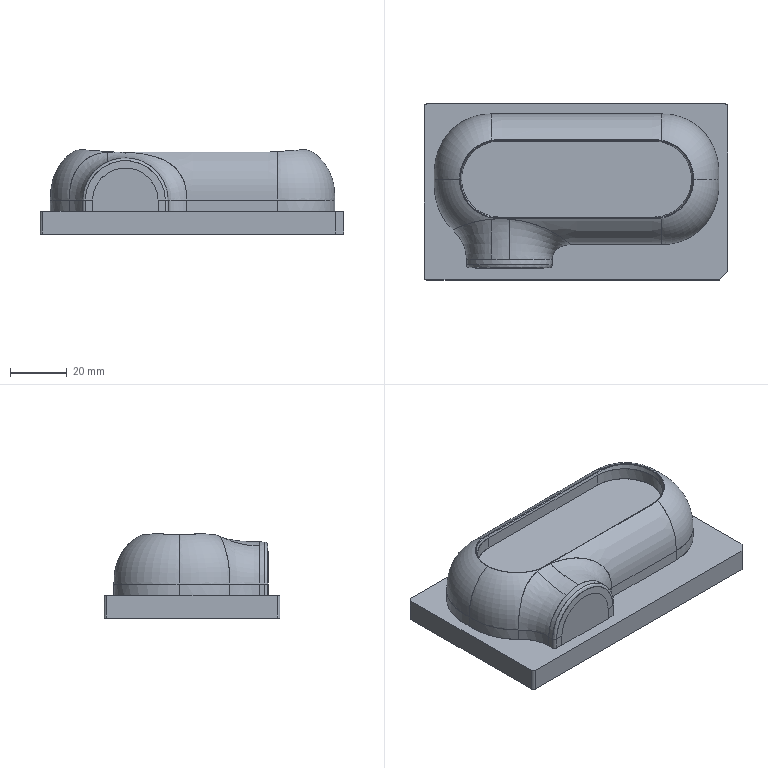NC program | PowerMill | posted by the shop | part box 107 x 62 x 29.663 mm
Lines 1 to 1401 of 415021:
%
G40 G49 G17 G80
( TOOL ID   D10C_1_1_1 )
( TOOL DIA. 10. TIP RAD 0 LENGTH 85.12 )
( Z = -.028 )
T1 M6
T3
G91 G28 Z0
G0 G90 G54
M08
S8000 M3
G0 X0 Y0 M8
G43 Z10.2 H1
X61.32 Y33.82
Z1.172
G1 Z-.028 F6000
X56.32 F10000
X-56.32
Y28.183
X56.32
Y22.547
X-56.32
Y16.91
X56.32
Y11.273
X-56.32
Y5.637
X56.32
Y0
X-56.32
Y-5.637
X56.32
Y-11.273
X-56.32
Y-16.91
X56.32
Y-22.547
X-56.32
Y-28.183
X56.32
Y-33.82
X-56.32
X-61.32
G0 Z10.2
X.218 Y.346
Z9.922
X-63.011 Y-.592
Z.741
G1 Z-.459 F6000
X-62.484 F10000
G3 X-57.736 Y4.155 I0 J4.747
G1 Y34.32
G2 X-56.736 Y35.32 I1. J0
G1 X57.172
G2 X58.172 Y34.32 I0 J-1.
G1 Y4.157
X46.989 Y4.213
X46.981 Y2.666
X46.858 Y1.119
X46.75 Y.346
X46.444 Y-1.201
X46.234 Y-1.974
X45.989 Y-2.748
X45.705 Y-3.521
X45.379 Y-4.295
X44.69 Y-5.67
X43.917 Y-6.909
X43.143 Y-7.943
X42.37 Y-8.824
X41.464 Y-9.709
X40.538 Y-10.482
X39.276 Y-11.364
X38.103 Y-12.029
X36.956 Y-12.564
X36.336 Y-12.802
X35.409 Y-13.113
X34.635 Y-13.324
X33.862 Y-13.484
X33.089 Y-13.541
X32.315 Y-13.482
X31.542 Y-13.336
X30.768 Y-13.065
X30.255 Y-12.802
X29.995 Y-12.641
X29.221 Y-12.006
X28.448 Y-11.061
X28.137 Y-10.482
X27.854 Y-9.709
X27.701 Y-8.935
X27.663 Y-8.162
X27.738 Y-7.388
X27.938 Y-6.615
X28.277 Y-5.841
X28.448 Y-5.53
X28.775 Y-5.068
X29.221 Y-4.565
X29.519 Y-4.295
X29.995 Y-3.932
X30.618 Y-3.521
X31.542 Y-2.947
X32.315 Y-2.422
X33.089 Y-1.791
X33.676 Y-1.201
X34.287 Y-.427
X34.635 Y.09
X35.16 Y1.119
X35.409 Y1.758
X35.658 Y2.666
X35.791 Y3.44
X35.867 Y4.213
X35.856 Y4.987
X35.767 Y5.76
X35.614 Y6.533
X35.386 Y7.307
X35.076 Y8.08
X34.67 Y8.854
X34.149 Y9.627
X33.488 Y10.401
X33.089 Y10.791
X32.315 Y11.421
X31.542 Y11.949
X31.531 Y11.956
X30.768 Y12.422
X29.995 Y12.931
X29.296 Y13.494
X28.632 Y14.268
X28.448 Y14.531
X28.326 Y14.758
X23.408 Y12.411
X18.896 Y10.258
X13.458 Y8.694
X7.5 Y6.981
X2.145 Y5.441
G3 X.47 Y6.699 I-1.67 J-.48
G1 X-.091 Y6.697
G3 X-1.804 Y4.698 I.005 J-1.738
G1 X-.811 Y-1.952
G3 X1.364 Y-1.929 I1.086 J.159
G1 X2.2 Y4.745
G3 X2.145 Y5.441 I-1.724 J.216
G1 X7.5 Y6.981
X6.371 Y11.317
G3 X4.434 Y12.813 I-1.935 J-.504
G1 X-4.065 Y12.807
G3 X-6.001 Y11.304 I.001 J-2.
G1 X-7.581 Y5.143
G3 X-7.603 Y4.242 I1.937 J-.497
G1 X-6.958 Y1.11
G2 X-5.807 Y-7.803 I-58.994 J-12.149
G1 X-5.648 Y-10.764
G3 X-3.648 Y-12.657 I1.997 J.107
G1 X4.075 Y-12.647
G3 X6.072 Y-10.669 I-.003 J2.
G1 X6.082 Y-9.832
G2 X6.632 Y-4.073 I34.451 J-.385
G1 X8.091 Y3.977
G3 X8.058 Y4.837 I-1.968 J.357
G1 X7.5 Y6.981
X13.458 Y8.694
X13.328 Y9.066
G2 X11.725 Y15.34 I35.2 J12.336
G1 X11.424 Y17.169
G3 X9.45 Y18.844 I-1.973 J-.325
G1 X-9.045 Y18.838
G3 X-11.014 Y17.186 I.001 J-2.
G1 X-11.379 Y15.118
G2 X-12.836 Y9.467 I-37.025 J6.534
G1 X-14.269 Y5.285
G3 X-14.267 Y3.984 I1.892 J-.648
G1 X-12.599 Y-.845
G2 X-12.515 Y-15.174 I-21.097 J-7.289
G1 X-12.73 Y-15.823
G3 X-10.831 Y-18.454 I1.898 J-.631
G1 X11.141 Y-18.441
G3 X13.074 Y-15.933 I-.001 J2.
G1 X12.52 Y-13.822
G2 X12.157 Y-4.693 I20.543 J5.389
G1 X12.185 Y-4.537
G2 X12.999 Y-1.397 I20.789 J-3.718
G1 X14.751 Y3.705
G3 X14.747 Y5.016 I-1.892 J.65
G1 X13.458 Y8.694
X18.896 Y10.258
G2 X19.274 Y24.679 I14.332 J6.839
G1 X19.284 Y24.697
Y24.699
X19.282 Y24.7
X-18.832
X-18.834 Y24.699
Y24.697
X-18.825 Y24.679
X-18.78 Y24.596
X-18.736 Y24.512
X-18.735 Y24.51
G2 X-23.208 Y4.655 I-13.944 J-7.29
G1 X-23.224 Y4.643
X-23.225 Y4.641
X-23.224 Y4.639
X-23.21 Y4.628
G2 X-39.737 Y-22.434 I-9.627 J-12.698
G1 X-41.719 Y-21.482
G2 X-47.231 Y-17.93 I11.424 J23.781
G1 X-47.249 Y-17.915
X-47.25
X-47.251 Y-17.917
X-47.16 Y-24.004
X-47.159 Y-24.007
X-47.157 Y-24.008
X30.537
X30.538 Y-24.007
Y-24.005
X30.52 Y-24.002
G2 X23.708 Y-21.091 I2.631 J15.581
X17.688 Y-5.165 I9.443 J12.67
G1 X17.714 Y-5.041
G2 X23.758 Y4.324 I15.259 J-3.214
G1 X23.773 Y4.335
X23.774 Y4.337
X23.773 Y4.339
X23.756 Y4.351
G2 X18.896 Y10.258 I9.472 J12.746
G1 X23.408 Y12.411
G3 X27.403 Y7.907 I9.82 J4.686
G1 X27.843 Y7.628
G2 X27.815 Y1.013 I-2.091 J-3.299
G1 X27.377 Y.74
G3 X22.606 Y-6.072 I5.597 J-8.996
G1 X22.58 Y-6.195
G3 X38.305 Y-17.914 I10.57 J-2.227
G1 X40.991 Y-16.456
G3 X50.325 Y-6.291 I-10.147 J18.686
G1 X50.81 Y-5.184
G2 X52.872 Y-5.631 I.986 J-.431
G1 X52.551 Y-27.037
G2 X50.551 Y-29.007 I-2. J.03
G1 X41.678
Y-24.008
X35.763
X35.762 Y-24.007
X35.763 Y-24.005
X35.781 Y-24.002
G3 X40.691 Y-22.308 I-2.63 J15.581
G1 X43.377 Y-20.849
G3 X47.665 Y-17.938 I-12.532 J23.079
G1 X47.685 Y-17.922
X47.687
Y-17.924
X47.596 Y-24.004
X47.595 Y-24.007
X47.593 Y-24.008
X41.678
Y-29.007
X-50.115
G2 X-52.115 Y-27.037 I0 J2.
G1 X-52.436 Y-5.602
G2 X-50.373 Y-5.155 I1.076 J.016
G1 X-49.889 Y-6.262
G3 X-39.554 Y-16.976 I19.595 J8.562
G1 X-37.573 Y-17.927
G3 X-27.019 Y1.189 I4.735 J9.857
G1 X-27.459 Y1.466
G2 X-27.446 Y7.832 I1.998 J3.179
G1 X-27.007 Y8.105
G3 X-36.928 Y27.079 I-5.673 J9.115
G1 X-38.994 Y26.189
G3 X-49.886 Y15.391 I8.303 J-19.269
G1 X-50.373 Y14.289
G2 X-52.436 Y14.75 I-.986 J.435
G1 X-52.114 Y27.748
G2 X-50.115 Y29.699 I1.999 J-.049
G1 X50.551
G2 X52.55 Y27.748 I0 J-2.
G1 X52.872 Y14.743
G2 X50.796 Y14.265 I-1.087 J-.027
G1 X50.292 Y15.37
G3 X39.827 Y26.007 I-19.831 J-9.045
G1 X37.903 Y26.922
G3 X23.408 Y12.411 I-4.676 J-9.825
G1 X28.326 Y14.758
X28.175 Y15.041
X27.876 Y15.815
X27.704 Y16.588
X27.675 Y16.908
Y17.76
X27.736 Y18.135
X27.91 Y18.908
X28.236 Y19.682
X28.448 Y20.04
X28.74 Y20.455
X29.221 Y21.02
X29.995 Y21.642
X30.642 Y22.002
X31.542 Y22.329
X32.315 Y22.477
X33.089 Y22.539
X33.862 Y22.483
X34.635 Y22.326
X35.76 Y22.002
X36.956 Y21.565
X37.729 Y21.21
X38.503 Y20.811
X39.125 Y20.455
X40.274 Y19.682
X41.238 Y18.908
X42.37 Y17.823
X43.143 Y16.942
X43.917 Y15.912
X44.69 Y14.673
X45.291 Y13.494
X45.463 Y13.102
X45.921 Y11.947
X46.392 Y10.401
X46.718 Y8.854
X46.914 Y7.307
X46.997 Y5.76
X46.989 Y4.213
X58.172 Y4.157
Y-33.628
G2 X57.172 Y-34.628 I-1. J0
G1 X-56.736
G2 X-57.736 Y-33.628 I0 J1.
G1 Y4.155
X-46.549 Y4.213
X-46.557 Y5.76
X-46.53 Y6.533
X-46.392 Y8.08
X-46.277 Y8.854
X-45.952 Y10.401
X-45.478 Y11.947
X-44.85 Y13.494
X-44.254 Y14.663
X-43.543 Y15.815
X-42.707 Y16.936
X-41.934 Y17.821
X-40.8 Y18.908
X-39.837 Y19.682
X-38.84 Y20.362
X-38.067 Y20.809
X-37.248 Y21.229
X-36.52 Y21.563
X-35.746 Y21.858
X-34.973 Y22.112
X-34.199 Y22.323
X-33.426 Y22.486
X-32.653 Y22.541
X-31.879 Y22.477
X-31.106 Y22.33
X-30.332 Y22.061
X-29.559 Y21.64
X-29.013 Y21.229
X-28.785 Y21.022
X-28.287 Y20.455
X-27.797 Y19.682
X-27.489 Y18.908
X-27.287 Y18.135
X-27.239 Y17.768
X-27.219 Y17.361
X-27.266 Y16.588
X-27.44 Y15.815
X-27.726 Y15.041
X-28.012 Y14.522
X-28.187 Y14.268
X-28.785 Y13.561
X-29.559 Y12.927
X-30.332 Y12.418
X-31.106 Y11.947
X-31.879 Y11.417
X-32.653 Y10.788
X-33.045 Y10.401
X-33.709 Y9.627
X-34.199 Y8.904
X-34.637 Y8.08
X-34.95 Y7.307
X-35.179 Y6.533
X-35.334 Y5.76
X-35.416 Y4.987
X-35.429 Y4.213
X-35.354 Y3.44
X-35.218 Y2.666
X-35.014 Y1.893
X-34.721 Y1.119
X-34.34 Y.346
X-33.848 Y-.427
X-33.235 Y-1.201
X-32.653 Y-1.787
X-31.879 Y-2.421
X-31.413 Y-2.748
X-31.401 Y-2.755
X-30.332 Y-3.417
X-29.559 Y-3.929
X-29.081 Y-4.295
X-28.785 Y-4.559
X-28.331 Y-5.068
X-28.012 Y-5.52
X-27.836 Y-5.841
X-27.503 Y-6.615
X-27.3 Y-7.388
X-27.239 Y-7.893
Y-8.788
X-27.418 Y-9.709
X-27.698 Y-10.482
X-28.012 Y-11.057
X-28.803 Y-12.029
X-29.559 Y-12.64
X-29.822 Y-12.802
X-30.332 Y-13.061
X-31.106 Y-13.333
X-31.879 Y-13.481
X-32.653 Y-13.537
X-33.426 Y-13.487
X-34.199 Y-13.325
X-34.973 Y-13.113
X-35.746 Y-12.86
X-36.52 Y-12.563
X-37.667 Y-12.029
X-38.84 Y-11.359
X-40.095 Y-10.482
X-41.025 Y-9.709
X-41.824 Y-8.935
X-42.707 Y-7.937
X-43.481 Y-6.907
X-44.254 Y-5.663
X-44.935 Y-4.295
X-45.262 Y-3.521
X-45.547 Y-2.748
X-46.003 Y-1.201
X-46.311 Y.346
X-46.494 Y1.893
X-46.541 Y2.666
X-46.549 Y4.213
X-57.736 Y4.155
G0 Z3.359
G1 X-63.011 Y-.592
G0 Z.359
G1 Z-.841 F6000
X-62.484 F10000
G3 X-57.736 Y4.155 I0 J4.747
G1 Y34.32
G2 X-56.736 Y35.32 I1. J0
G1 X57.172
G2 X58.172 Y34.32 I0 J-1.
G1 Y7.76
X47.549 Y7.307
X47.615 Y5.76
X47.605 Y2.666
X47.497 Y1.119
X47.266 Y-.427
X47.01 Y-1.612
X46.688 Y-2.748
X46.237 Y-4.013
X45.775 Y-5.068
X45.379 Y-5.841
X44.69 Y-7.014
X43.88 Y-8.162
X43.143 Y-9.059
X42.536 Y-9.709
X41.596 Y-10.591
X40.776 Y-11.255
X39.658 Y-12.029
X38.503 Y-12.696
X37.729 Y-13.074
X36.527 Y-13.576
X35.409 Y-13.946
X34.635 Y-14.156
X33.752 Y-14.349
X32.315 Y-14.543
X31.542 Y-14.61
X29.995 Y-14.666
X27.675 Y-14.648
X-8.676 Y-14.634
X-20.278 Y-14.637
X-26.465 Y-14.633
X-28.012 Y-14.669
X-30.332 Y-14.659
X-31.106 Y-14.62
X-31.879 Y-14.544
X-33.312 Y-14.349
X-34.199 Y-14.155
X-34.973 Y-13.947
X-35.746 Y-13.699
X-36.52 Y-13.407
X-37.863 Y-12.802
X-38.84 Y-12.263
X-39.613 Y-11.772
X-40.387 Y-11.218
X-41.16 Y-10.588
X-41.934 Y-9.873
X-42.707 Y-9.051
X-43.44 Y-8.162
X-44.254 Y-7.008
X-44.939 Y-5.841
X-45.337 Y-5.068
X-45.801 Y-4.007
X-46.252 Y-2.748
X-46.574 Y-1.595
X-46.827 Y-.427
X-47.057 Y1.119
X-47.125 Y1.893
X-47.176 Y3.44
X-47.156 Y6.533
X-47.034 Y8.08
X-46.791 Y9.627
X-46.622 Y10.401
X-46.182 Y11.947
X-45.912 Y12.721
X-45.236 Y14.268
X-44.834 Y15.041
X-44.375 Y15.815
X-43.865 Y16.588
X-43.287 Y17.361
X-42.707 Y18.054
X-41.934 Y18.873
X-41.16 Y19.589
X-40.387 Y20.218
X-39.613 Y20.772
X-38.84 Y21.263
X-38.067 Y21.694
X-37.448 Y22.002
X-36.52 Y22.408
X-35.746 Y22.697
X-34.973 Y22.947
X-34.199 Y23.153
X-33.426 Y23.324
X-31.818 Y23.549
X-30.332 Y23.652
X-28.012 Y23.669
X-26.465 Y23.642
X-26.461
X-14.864 Y23.636
X23.034 Y23.638
X27.675 Y23.661
X30.768 Y23.652
X32.256 Y23.549
X33.862 Y23.325
X34.635 Y23.156
X35.409 Y22.949
X36.182 Y22.698
X36.956 Y22.41
X37.729 Y22.075
X38.503 Y21.697
X39.276 Y21.264
X40.049 Y20.775
X40.501 Y20.455
X41.491 Y19.682
X42.337 Y18.908
X43.077 Y18.135
X43.73 Y17.361
X44.305 Y16.588
X44.69 Y16.013
X45.274 Y15.041
X45.676 Y14.268
X46.237 Y13.013
X46.625 Y11.947
X47.062 Y10.401
X47.368 Y8.854
X47.476 Y8.08
X47.549 Y7.307
X58.172 Y7.76
Y-33.628
G2 X57.172 Y-34.628 I-1. J0
G1 X-41.666
X-41.378 Y-29.401
X-41.112 Y-24.561
G3 X-40.628 Y-22.636 I.056 J1.009
G1 X-41.647 Y-22.16
G2 X-44.142 Y-20.821 I10.89 J23.293
G1 X-45.403 Y-20.053
G3 X-47.631 Y-21.659 I-.776 J-1.273
G1 X-47.377 Y-22.767
G3 X-45.538 Y-24.317 I1.95 J.447
G1 X-41.112 Y-24.561
X-41.378 Y-29.401
X-52.349
G2 X-52.509 Y-29.241 I0 J.16
G1 Y29.933
G2 X-52.349 Y30.093 I.16 J0
G1 X52.785
G2 X52.945 Y29.933 I0 J-.16
G1 Y12.931
G2 X52.784 Y12.763 I-.169 J0
G1 X52.009 Y12.73
G2 X51.79 Y12.888 I-.009 J.217
G1 X51.653 Y13.373
X51.598 Y13.555
X51.536 Y13.735
X51.148 Y14.8
X51.08 Y14.978
X51.005 Y15.153
X50.38 Y16.545
X50.283 Y16.739
X50.11 Y17.077
X49.932 Y17.413
X49.824 Y17.614
X49.136 Y18.761
X48.607 Y19.555
X48.492 Y19.716
X48.205 Y20.108
X47.911 Y20.496
X47.806 Y20.633
X47.694 Y20.77
X47.378 Y21.149
X47.056 Y21.523
X46.941 Y21.654
X46.823 Y21.782
X46.488 Y22.137
X46.147 Y22.486
X46.005 Y22.63
X45.958 Y22.677
X45.022 Y23.535
X44.868 Y23.67
X44.709 Y23.8
X43.671 Y24.61
X43.004 Y25.085
X42.944 Y25.126
X41.997 Y25.726
X41.935 Y25.764
X40.974 Y26.302
X40.91 Y26.336
X39.969 Y26.797
X38.923 Y27.252
X38.695 Y27.342
G3 X35.109 Y28.404 I-7.932 J-20.187
G1 X34.909 Y28.445
X34.747 Y28.475
X34.585 Y28.501
X32.979 Y28.725
X32.798 Y28.747
X32.618 Y28.763
X31.15 Y28.864
X30.922 Y28.876
X30.067 Y28.881
X28.893 Y28.885
X27.718 Y28.887
X-27.931 Y28.894
X-30.351 Y28.878
X-30.562 Y28.873
X-32.176 Y28.763
X-32.359 Y28.747
X-32.542 Y28.725
X-34.149 Y28.5
X-34.352 Y28.468
X-34.554 Y28.427
X-35.399 Y28.24
X-36.4 Y27.975
X-36.466 Y27.956
X-37.409 Y27.652
X-38.432 Y27.271
X-38.501 Y27.244
X-39.615 Y26.758
X-39.675 Y26.73
X-40.504 Y26.317
X-41.466 Y25.781
X-41.531 Y25.743
X-42.49 Y25.135
X-42.552 Y25.094
X-43.539 Y24.387
X-43.722 Y24.243
X-44.075 Y23.961
X-44.423 Y23.674
X-44.606 Y23.519
X-45.485 Y22.707
X-45.732 Y22.463
X-46.594 Y21.547
X-46.646 Y21.489
X-47.351 Y20.647
X-47.397 Y20.59
X-48.107 Y19.64
X-48.153 Y19.576
X-48.807 Y18.585
X-49.406 Y17.574
X-49.503 Y17.393
X-49.683 Y17.052
X-49.858 Y16.708
X-49.941 Y16.543
X-49.97 Y16.482
X-50.699 Y14.818
X-50.778 Y14.627
X-50.85 Y14.434
X-51.147 Y13.577
X-51.17 Y13.506
X-51.644 Y11.85
X-51.698 Y11.647
X-51.916 Y10.648
X-51.932 Y10.571
X-52.196 Y8.894
X-52.224 Y8.693
X-52.244 Y8.492
X-52.366 Y6.945
X-52.377 Y6.757
X-52.382 Y6.568
X-52.403 Y3.405
X-52.344 Y1.632
X-52.341 Y1.558
X-52.253 Y.563
X-52.244 Y.486
X-52. Y-1.175
X-51.972 Y-1.347
X-51.96 Y-1.411
X-51.66 Y-2.796
X-51.642 Y-2.871
X-51.286 Y-4.151
X-51.232 Y-4.331
X-51.172 Y-4.51
X-50.721 Y-5.768
X-50.669 Y-5.909
X-50.612 Y-6.047
X-50.512 Y-6.283
X-50.335 Y-6.693
X-50.153 Y-7.101
X-50.046 Y-7.334
X-49.544 Y-8.312
X-49.509 Y-8.377
X-48.763 Y-9.65
X-48.648 Y-9.838
X-48.525 Y-10.02
X-47.711 Y-11.174
X-47.613 Y-11.308
X-47.511 Y-11.439
X-47.349 Y-11.64
X-47.065 Y-11.989
X-46.775 Y-12.333
X-46.643 Y-12.489
X-46.6 Y-12.538
X-45.744 Y-13.45
X-45.635 Y-13.563
X-45.523 Y-13.672
X-45.347 Y-13.839
X-45.022 Y-14.141
X-44.694 Y-14.438
X-44.561 Y-14.557
X-44.425 Y-14.671
X-44.081 Y-14.955
X-43.733 Y-15.234
X-43.541 Y-15.386
X-42.582 Y-16.073
X-42.521 Y-16.115
X-41.582 Y-16.712
X-41.514 Y-16.753
X-40.398 Y-17.372
X-40.206 Y-17.474
X-40.009 Y-17.568
X-38.683 Y-18.165
X-38.488 Y-18.249
X-37.469 Y-18.633
X-36.512 Y-18.942
X-35.496 Y-19.218
X-34.441 Y-19.452
X-34.23 Y-19.494
X-34.017 Y-19.528
X-32.583 Y-19.722
X-31.558 Y-19.827
X-30.536 Y-19.882
X-28.062 Y-19.896
X30.037 Y-19.892
X31.812 Y-19.829
X31.878 Y-19.826
X32.829 Y-19.744
X34.443 Y-19.53
X34.658 Y-19.496
X34.872 Y-19.454
X35.829 Y-19.244
X35.893 Y-19.229
X36.865 Y-18.965
X36.934 Y-18.945
X38.167 Y-18.538
X38.357 Y-18.471
X38.544 Y-18.397
X39.832 Y-17.858
X39.901 Y-17.828
X40.79 Y-17.395
X40.954 Y-17.312
X41.116 Y-17.222
X42.272 Y-16.555
X42.454 Y-16.444
X42.632 Y-16.327
X43.189 Y-15.941
X45.824 Y-20.012
G2 X48.041 Y-21.477 I.789 J-1.216
G1 X47.834 Y-22.663
G2 X45.973 Y-24.317 I-1.97 J.343
G1 X41.514 Y-24.561
G2 X41.031 Y-22.634 I-.055 J1.01
G1 X42.041 Y-22.163
G3 X44.33 Y-20.955 I-11.165 J23.93
G1 X44.761 Y-20.7
X45.824 Y-20.012
X43.189 Y-15.941
X43.75 Y-15.553
X43.909 Y-15.439
X44.064 Y-15.318
X44.884 Y-14.654
X45.009 Y-14.55
X45.131 Y-14.441
X45.332 Y-14.257
X45.729 Y-13.887
X46.121 Y-13.511
X46.26 Y-13.375
X46.379 Y-13.252
X46.659 Y-12.956
X46.935 Y-12.656
X47.091 Y-12.484
X47.916 Y-11.482
X48.036 Y-11.331
X48.15 Y-11.175
X48.96 Y-10.027
X49.083 Y-9.845
X49.198 Y-9.657
X49.932 Y-8.407
X49.969 Y-8.34
X50.471 Y-7.36
X50.505 Y-7.29
X51.021 Y-6.117
X51.082 Y-5.973
X51.138 Y-5.828
X51.235 Y-5.565
X51.428 Y-5.032
X51.613 Y-4.496
X51.677 Y-4.306
X51.733 Y-4.119
X51.881 Y-3.611
X52.021 Y-3.101
X52.087 Y-2.853
X52.371 Y-1.552
X52.413 Y-1.335
X52.666 Y.345
X52.692 Y.546
X52.71 Y.748
X52.816 Y2.224
X52.832 Y2.257
X52.866 Y2.269
X52.898 Y2.268
X52.932 Y2.253
X52.945 Y2.219
Y-29.241
G2 X52.785 Y-29.401 I-.16 J0
G1 X-41.378
X-41.666 Y-34.628
X-56.736
G2 X-57.736 Y-33.628 I0 J1.
G1 Y4.155
G0 Z2.978
G1 X-63.011 Y-.592
G0 Z-.022
G1 Z-1.222 F6000
X-62.484 F10000
G3 X-57.736 Y4.155 I0 J4.747
G1 Y34.32
G2 X-56.736 Y35.32 I1. J0
G1 X57.172
G2 X58.172 Y34.32 I0 J-1.
G1 Y7.323
X48.101 Y6.92
X48.147 Y5.76
X48.136 Y2.666
X48.035 Y1.119
X47.831 Y-.427
X47.5 Y-1.974
X47.283 Y-2.748
X47.03 Y-3.521
X46.741 Y-4.295
X46.237 Y-5.446
X45.463 Y-6.891
X44.69 Y-8.087
X44.049 Y-8.935
X43.389 Y-9.709
X42.64 Y-10.482
X41.785 Y-11.255
X40.823 Y-12.01
X40.049 Y-12.543
X39.63 Y-12.802
X38.503 Y-13.432
X37.729 Y-13.797
X36.324 Y-14.349
X35.409 Y-14.636
X34.635 Y-14.842
X33.862 Y-15.008
X33.178 Y-15.123
X32.315 Y-15.239
X31.542 Y-15.308
X30.768 Y-15.34
X-18.731 Y-15.347
X-18.736
X-21.825 Y-15.409
X-24.145 Y-15.444
X-30.332 Y-15.389
X-31.106 Y-15.342
X-32.653 Y-15.152
X-34.199 Y-14.843
X-34.973 Y-14.64
X-35.887 Y-14.349
X-36.52 Y-14.114
X-37.766 Y-13.576
X-38.84 Y-13.012
X-39.613 Y-12.54
X-40.387 Y-12.006
X-41.347 Y-11.255
X-41.934 Y-10.73
X-42.707 Y-9.961
X-43.608 Y-8.935
X-44.254 Y-8.082
X-45.027 Y-6.881
X-45.801 Y-5.438
X-46.3 Y-4.295
X-46.574 Y-3.571
X-46.845 Y-2.748
X-47.06 Y-1.974
X-47.24 Y-1.201
X-47.511 Y.346
X-47.596 Y1.119
X-47.696 Y2.666
X-47.708 Y5.76
X-47.646 Y7.307
X-47.483 Y8.854
X-47.348 Y9.67
X-47.196 Y10.401
X-46.782 Y11.947
X-46.216 Y13.494
X-45.881 Y14.268
X-45.499 Y15.041
X-45.027 Y15.885
X-44.254 Y17.081
X-43.481 Y18.088
X-42.707 Y18.963
X-41.934 Y19.729
X-41.16 Y20.407
X-40.387 Y21.007
X-39.613 Y21.54
X-38.84 Y22.013
X-38.067 Y22.431
X-37.293 Y22.796
X-36.52 Y23.116
X-35.276 Y23.549
X-34.199 Y23.841
X-33.426 Y24.008
X-31.879 Y24.238
X-30.857 Y24.322
X-28.785 Y24.343
X29.221 Y24.345
X31.329 Y24.322
X32.315 Y24.239
X33.862 Y24.008
X34.635 Y23.842
X35.718 Y23.549
X36.956 Y23.117
X37.729 Y22.797
X38.503 Y22.433
X39.301 Y22.002
X40.049 Y21.543
X40.513 Y21.229
X41.596 Y20.41
X42.426 Y19.682
X43.199 Y18.908
X43.88 Y18.135
X44.69 Y17.085
X45.463 Y15.891
X45.937 Y15.041
X46.237 Y14.448
X46.661 Y13.494
X47.01 Y12.584
X47.446 Y11.174
X47.784 Y9.693
X47.925 Y8.854
X48.085 Y7.307
X48.101 Y6.92
X58.172 Y7.323
Y-33.628
G2 X57.172 Y-34.628 I-1. J0
G1 X-42.227
X-41.933 Y-29.639
X-41.648 Y-24.798
G3 X-41.137 Y-22.858 I.06 J1.021
G1 X-42.161 Y-22.357
X-43.282 Y-21.774
X-44.374 Y-21.139
X-45.635 Y-20.365
G3 X-47.864 Y-21.991 I-.78 J-1.271
G1 X-47.608 Y-23.034
G3 X-45.784 Y-24.554 I1.942 J.476
G1 X-41.648 Y-24.798
X-41.933 Y-29.639
X-52.671
X-52.725 Y-29.617
X-52.747 Y-29.563
Y30.255
X-52.725 Y30.309
X-52.671 Y30.331
X53.107
X53.161 Y30.309
X53.183 Y30.255
Y12.194
X53.161 Y12.139
X53.106 Y12.114
X52.436 Y12.087
X52.373 Y12.107
X52.337 Y12.163
X52.307 Y12.292
X52.263 Y12.47
X52.212 Y12.646
X51.777 Y14.056
X51.725 Y14.213
X51.668 Y14.369
X51.319 Y15.28
X51.271 Y15.402
X51.219 Y15.522
X50.795 Y16.476
X50.742 Y16.59
X50.687 Y16.703
X50.36 Y17.347
X50.336 Y17.393
X49.822 Y18.317
X49.739 Y18.461
X49.651 Y18.602
X48.878 Y19.797
X48.762 Y19.967
X48.64 Y20.132
X47.831 Y21.181
X47.729 Y21.309
X47.624 Y21.432
X46.943 Y22.206
X46.836 Y22.322
X46.727 Y22.436
X45.953 Y23.209
X45.838 Y23.321
X45.718 Y23.43
X44.889 Y24.158
X44.748 Y24.277
X44.604 Y24.391
X43.521 Y25.209
X43.432 Y25.274
X43.342 Y25.338
X43.223 Y25.42
X43.046 Y25.541
X42.867 Y25.66
X42.769 Y25.725
X42.73 Y25.75
X41.913 Y26.253
X41.792 Y26.324
X41.669 Y26.393
X40.87 Y26.824
X40.769 Y26.877
X40.667 Y26.927
X40.501 Y27.007
X40.2 Y27.151
X39.897 Y27.291
X39.763 Y27.352
X39.719 Y27.372
X38.868 Y27.725
X38.734 Y27.779
X38.598 Y27.828
X37.361 Y28.259
X37.192 Y28.315
X37.021 Y28.364
X35.938 Y28.657
X35.813 Y28.69
X35.686 Y28.719
X34.913 Y28.885
X34.756 Y28.916
X34.598 Y28.943
X33.052 Y29.173
X32.893 Y29.194
X32.733 Y29.21
X31.747 Y29.293
X31.565 Y29.305
X31.383 Y29.311
X29.287 Y29.334
X-28.776 Y29.332
X-30.907 Y29.311
X-31.087 Y29.306
X-31.266 Y29.294
X-32.289 Y29.21
X-32.452 Y29.194
X-32.614 Y29.172
X-34.161 Y28.942
X-34.32 Y28.916
X-34.477 Y28.884
X-35.251 Y28.718
X-35.379 Y28.688
X-35.506 Y28.655
X-36.582 Y28.363
X-36.75 Y28.315
X-36.916 Y28.26
X-38.16 Y27.827
X-38.294 Y27.778
X-38.426 Y27.726
X-39.2 Y27.406
X-39.312 Y27.358
X-39.423 Y27.307
X-40.196 Y26.942
X-40.317 Y26.883
X-40.436 Y26.821
X-41.209 Y26.404
X-41.328 Y26.338
X-41.445 Y26.268
X-42.218 Y25.795
X-42.332 Y25.723
X-42.444 Y25.648
X-43.217 Y25.115
X-43.332 Y25.033
X-43.445 Y24.948
X-44.219 Y24.348
X-44.335 Y24.255
X-44.448 Y24.159
X-45.221 Y23.482
X-45.335 Y23.379
X-45.445 Y23.273
X-46.218 Y22.507
X-46.334 Y22.389
X-46.445 Y22.267
X-47.218 Y21.392
X-47.33 Y21.261
X-47.437 Y21.126
X-48.211 Y20.119
X-48.33 Y19.957
X-48.443 Y19.79
X-49.216 Y18.594
X-49.302 Y18.457
X-49.384 Y18.316
X-49.855 Y17.472
X-49.914 Y17.363
X-49.971 Y17.252
X-50.353 Y16.478
X-50.408 Y16.365
X-50.459 Y16.249
X-50.794 Y15.476
X-50.849 Y15.343
X-50.9 Y15.209
X-51.467 Y13.662
X-51.538 Y13.452
X-51.601 Y13.239
X-52.015 Y11.692
X-52.051 Y11.551
X-52.082 Y11.409
X-52.244 Y10.623
X-52.254 Y10.573
X-52.404 Y9.674
X-52.427 Y9.524
X-52.445 Y9.374
X-52.607 Y7.827
X-52.621 Y7.667
X-52.63 Y7.507
X-52.692 Y5.973
X-52.696 Y5.831
X-52.685 Y2.649
X-52.682 Y2.496
X-52.674 Y2.344
X-52.575 Y.81
X-52.564 Y.667
X-52.471 Y-.193
X-52.45 Y-.354
X-52.425 Y-.514
X-52.154 Y-2.061
X-52.128 Y-2.2
X-52.098 Y-2.337
X-51.903 Y-3.17
X-51.89 Y-3.223
X-51.654 Y-4.072
X-51.612 Y-4.216
X-51.318 Y-5.114
X-51.271 Y-5.253
X-50.966 Y-6.06
X-50.92 Y-6.175
X-50.872 Y-6.29
X-50.373 Y-7.433
X-50.289 Y-7.616
X-50.198 Y-7.795
X-49.424 Y-9.238
X-49.326 Y-9.412
X-49.221 Y-9.582
X-48.448 Y-10.783
X-48.343 Y-10.94
X-48.231 Y-11.093
X-47.585 Y-11.946
X-47.474 Y-12.088
X-47.357 Y-12.226
X-46.457 Y-13.252
X-46.342 Y-13.378
X-46.223 Y-13.501
X-45.45 Y-14.269
X-45.357 Y-14.359
X-45.262 Y-14.446
X-44.675 Y-14.971
X-44.549 Y-15.081
X-44.419 Y-15.186
X-43.459 Y-15.936
X-43.342 Y-16.025
X-43.223 Y-16.11
X-42.449 Y-16.644
X-42.332 Y-16.723
X-42.213 Y-16.798
X-41.44 Y-17.27
X-41.3 Y-17.353
X-41.157 Y-17.43
X-40.083 Y-17.994
X-39.915 Y-18.078
X-39.744 Y-18.156
X-38.498 Y-18.694
X-38.378 Y-18.744
X-38.257 Y-18.79
X-37.624 Y-19.026
X-37.512 Y-19.066
X-37.398 Y-19.103
X-36.485 Y-19.394
X-36.362 Y-19.431
X-36.239 Y-19.465
X-35.465 Y-19.668
X-35.323 Y-19.703
X-35.179 Y-19.734
X-33.633 Y-20.044
X-33.446 Y-20.078
X-33.259 Y-20.104
X-31.712 Y-20.294
X-31.561 Y-20.31
X-31.409 Y-20.321
X-30.635 Y-20.368
X-30.506 Y-20.375
X-30.377 Y-20.377
X-24.149 Y-20.433
X-18.7 Y-20.358
X30.832 Y-20.328
X30.885
X31.743 Y-20.293
X31.844 Y-20.288
X31.946 Y-20.281
X32.118 Y-20.267
X32.417 Y-20.241
X32.715 Y-20.213
X32.855 Y-20.199
X32.901 Y-20.194
X33.902 Y-20.058
X34.023 Y-20.04
X34.336 Y-19.989
X34.649 Y-19.935
X34.781 Y-19.911
X34.827 Y-19.903
X35.681 Y-19.72
X35.78 Y-19.698
X35.879 Y-19.673
X36.048 Y-19.63
X36.347 Y-19.551
X36.645 Y-19.47
X36.813 Y-19.423
X37.815 Y-19.11
X37.983 Y-19.054
X38.149 Y-18.992
X39.554 Y-18.44
X39.707 Y-18.377
X39.858 Y-18.309
X40.632 Y-17.944
X40.785 Y-17.868
X40.935 Y-17.788
X42.051 Y-17.165
X42.178 Y-17.091
X42.672 Y-16.787
X42.777 Y-16.72
X42.88 Y-16.651
X43.286 Y-16.371
X45.938 Y-20.421
X46.061 Y-20.341
G2 X48.277 Y-21.821 I.795 J-1.21
G1 X48.066 Y-22.931
G2 X46.219 Y-24.554 I-1.965 J.373
G1 X42.08 Y-24.798
G2 X41.572 Y-22.859 I-.06 J1.02
G1 X42.582 Y-22.367
X43.629 Y-21.827
X44.652 Y-21.241
X45.081 Y-20.982
X45.938 Y-20.421
X43.286 Y-16.371
X43.653 Y-16.118
X43.778 Y-16.029
X43.9 Y-15.936
X44.863 Y-15.182
X45. Y-15.07
X45.133 Y-14.954
X45.988 Y-14.181
X46.108 Y-14.068
X46.225 Y-13.951
X46.973 Y-13.178
X47.08 Y-13.064
X47.183 Y-12.947
X47.843 Y-12.174
X47.937 Y-12.061
X48.027 Y-11.945
X48.669 Y-11.097
X48.777 Y-10.948
X48.879 Y-10.796
X49.653 Y-9.6
X49.761 Y-9.425
X49.862 Y-9.245
X50.635 Y-7.8
X50.725 Y-7.624
X50.808 Y-7.445
X51.311 Y-6.294
X51.364 Y-6.168
X51.414 Y-6.04
X51.724 Y-5.21
X51.738 Y-5.171
X51.751 Y-5.132
X52.044 Y-4.237
X52.06 Y-4.185
X52.302 Y-3.33
X52.343 Y-3.174
X52.379 Y-3.018
X52.71 Y-1.471
X52.747 Y-1.276
X52.777 Y-1.08
X52.981 Y.467
X53. Y.625
X53.013 Y.784
X53.1 Y2.083
X53.114 Y2.109
X53.141 Y2.116
X53.151 Y2.115
X53.173 Y2.103
X53.181 Y2.08
X53.183 Y-29.563
X53.161 Y-29.617
X53.107 Y-29.639
X-41.933
X-42.227 Y-34.628
X-56.736
G2 X-57.736 Y-33.628 I0 J1.
G1 Y4.155
G0 Z2.597
G1 X-63.011 Y-.592
G0 Z-.403
G1 Z-1.603 F6000
X-62.484 F10000
G3 X-57.736 Y4.155 I0 J4.747
G1 Y34.32
G2 X-56.736 Y35.32 I1. J0
G1 X.218
Y30.46
X52.347
G2 X53.312 Y29.495 I0 J-.965
G1 X53.313 Y12.552
G2 X52.681 Y12.471 I-.321 J0
G1 X52.588 Y12.823
G3 X30.524 Y29.822 I-22.061 J-5.817
G1 X-30.366 Y29.811
X-30.613 Y29.806
G3 X-45.823 Y23.535 I.505 J-22.805
G1 X-46.002 Y23.364
X-46.227 Y23.137
G3 X-52.119 Y12.91 I16.789 J-16.483
G1 X-52.243 Y12.459
G2 X-52.877 Y12.545 I-.311 J.086
G1 X-52.876 Y29.495
G2 X-51.911 Y30.46 I.965 J0
G1 X.218
Y35.32
X57.172
G2 X58.172 Y34.32 I0 J-1.
G1 Y6.552
X48.652 Y6.533
X48.66 Y2.666
X48.56 Y1.119
X48.359 Y-.427
X48.047 Y-1.974
X47.784 Y-2.945
X47.318 Y-4.295
X47.01 Y-5.06
X46.653 Y-5.841
X46.259 Y-6.615
X45.814 Y-7.388
X45.463 Y-7.94
X44.69 Y-9.033
X44.14 Y-9.709
X43.143 Y-10.799
X42.37 Y-11.524
X41.596 Y-12.166
X40.729 Y-12.802
X39.504 Y-13.576
X38.503 Y-14.104
X37.979 Y-14.349
X36.956 Y-14.772
X35.941 Y-15.123
X35.409 Y-15.276
X33.862 Y-15.646
X33.089 Y-15.763
X31.88 Y-15.896
X30.768 Y-15.954
X29.221 Y-15.959
X-11.77
X-17.184 Y-15.987
X-18.731 Y-16.083
X-18.742 Y-16.085
X-20.278 Y-16.25
X-22.598 Y-16.435
X-24.145 Y-16.483
X-25.692 Y-16.45
X-30.332 Y-16.16
X-31.879 Y-15.981
X-32.653 Y-15.85
X-34.199 Y-15.503
X-35.523 Y-15.123
X-36.52 Y-14.771
X-37.293 Y-14.462
X-38.067 Y-14.103